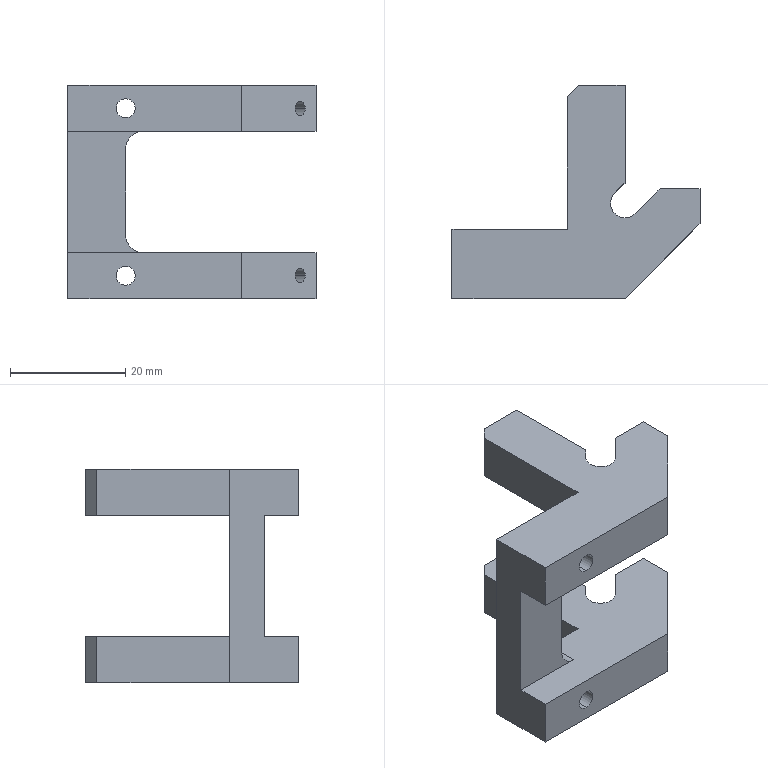Part | NX | features BREP 1 | 1 solid | 42 faces | box 43 x 37 x 37 mm | volume 12861 mm3 | plane 28 | cylinder 14 | commonest cylinder face diameters 2.5 x4 3.3 x4 5.05 x4 6 x2
STEP:
#1=CARTESIAN_POINT('',(-10.,0.,16.15));
#2=VERTEX_POINT('',#1);
#3=CARTESIAN_POINT('',(-10.,-12.,16.15));
#4=VERTEX_POINT('',#3);
#5=CARTESIAN_POINT('',(-10.,-12.,16.15));
#6=DIRECTION('',(0.,-1.,0.));
#7=VECTOR('',#6,1000.);
#8=LINE('',#5,#7);
#9=EDGE_CURVE('',#2,#4,#8,.T.);
#10=ORIENTED_EDGE('',*,*,#9,.F.);
#11=CARTESIAN_POINT('',(-10.,0.,12.85));
#12=VERTEX_POINT('',#11);
#13=CARTESIAN_POINT('',(-10.,0.,14.5));
#14=DIRECTION('',(0.,-1.,0.));
#15=DIRECTION('',(0.,0.,-1.));
#16=AXIS2_PLACEMENT_3D('',#13,#14,#15);
#17=CIRCLE('',#16,1.65);
#18=EDGE_CURVE('',#12,#2,#17,.T.);
#19=ORIENTED_EDGE('',*,*,#18,.F.);
#20=CARTESIAN_POINT('',(-10.,-12.,12.85));
#21=VERTEX_POINT('',#20);
#22=CARTESIAN_POINT('',(-10.,-12.,12.85));
#23=DIRECTION('',(0.,-1.,0.));
#24=VECTOR('',#23,1000.);
#25=LINE('',#22,#24);
#26=EDGE_CURVE('',#12,#21,#25,.T.);
#27=ORIENTED_EDGE('',*,*,#26,.T.);
#28=CARTESIAN_POINT('',(-10.,-12.,14.5));
#29=DIRECTION('',(0.,-1.,0.));
#30=DIRECTION('',(0.,0.,-1.));
#31=AXIS2_PLACEMENT_3D('',#28,#29,#30);
#32=CIRCLE('',#31,1.65);
#33=EDGE_CURVE('',#21,#4,#32,.T.);
#34=ORIENTED_EDGE('',*,*,#33,.T.);
#35=EDGE_LOOP('',(#10,#19,#27,#34));
#36=FACE_BOUND('',#35,.T.);
#37=CARTESIAN_POINT('',(-10.,-12.,14.5));
#38=DIRECTION('',(0.,-1.,0.));
#39=DIRECTION('',(0.,0.,-1.));
#40=AXIS2_PLACEMENT_3D('',#37,#38,#39);
#41=CYLINDRICAL_SURFACE('',#40,1.65);
#42=ADVANCED_FACE('',(#36),#41,.F.);
#43=CARTESIAN_POINT('',(-10.,0.,-12.85));
#44=VERTEX_POINT('',#43);
#45=CARTESIAN_POINT('',(-10.,-12.,-12.85));
#46=VERTEX_POINT('',#45);
#47=CARTESIAN_POINT('',(-10.,-12.,-12.85));
#48=DIRECTION('',(0.,-1.,0.));
#49=VECTOR('',#48,1000.);
#50=LINE('',#47,#49);
#51=EDGE_CURVE('',#44,#46,#50,.T.);
#52=ORIENTED_EDGE('',*,*,#51,.F.);
#53=CARTESIAN_POINT('',(-10.,0.,-16.15));
#54=VERTEX_POINT('',#53);
#55=CARTESIAN_POINT('',(-10.,0.,-14.5));
#56=DIRECTION('',(0.,-1.,0.));
#57=DIRECTION('',(0.,0.,-1.));
#58=AXIS2_PLACEMENT_3D('',#55,#56,#57);
#59=CIRCLE('',#58,1.65);
#60=EDGE_CURVE('',#54,#44,#59,.T.);
#61=ORIENTED_EDGE('',*,*,#60,.F.);
#62=CARTESIAN_POINT('',(-10.,-12.,-16.15));
#63=VERTEX_POINT('',#62);
#64=CARTESIAN_POINT('',(-10.,-12.,-16.15));
#65=DIRECTION('',(0.,-1.,0.));
#66=VECTOR('',#65,1000.);
#67=LINE('',#64,#66);
#68=EDGE_CURVE('',#54,#63,#67,.T.);
#69=ORIENTED_EDGE('',*,*,#68,.T.);
#70=CARTESIAN_POINT('',(-10.,-12.,-14.5));
#71=DIRECTION('',(0.,-1.,0.));
#72=DIRECTION('',(0.,0.,-1.));
#73=AXIS2_PLACEMENT_3D('',#70,#71,#72);
#74=CIRCLE('',#73,1.65);
#75=EDGE_CURVE('',#63,#46,#74,.T.);
#76=ORIENTED_EDGE('',*,*,#75,.T.);
#77=EDGE_LOOP('',(#52,#61,#69,#76));
#78=FACE_BOUND('',#77,.T.);
#79=CARTESIAN_POINT('',(-10.,-12.,-14.5));
#80=DIRECTION('',(0.,-1.,0.));
#81=DIRECTION('',(0.,0.,-1.));
#82=AXIS2_PLACEMENT_3D('',#79,#80,#81);
#83=CYLINDRICAL_SURFACE('',#82,1.65);
#84=ADVANCED_FACE('',(#78),#83,.F.);
#85=CARTESIAN_POINT('',(-10.,-6.,7.5));
#86=VERTEX_POINT('',#85);
#87=CARTESIAN_POINT('',(-7.,-6.,10.5));
#88=VERTEX_POINT('',#87);
#89=CARTESIAN_POINT('',(-7.,-6.,7.5));
#90=DIRECTION('',(0.,1.,0.));
#91=DIRECTION('',(1.,0.,0.));
#92=AXIS2_PLACEMENT_3D('',#89,#90,#91);
#93=CIRCLE('',#92,3.);
#94=EDGE_CURVE('',#86,#88,#93,.T.);
#95=ORIENTED_EDGE('',*,*,#94,.T.);
#96=CARTESIAN_POINT('',(-20.,-6.,10.5));
#97=VERTEX_POINT('',#96);
#98=CARTESIAN_POINT('',(-20.,-6.,10.5));
#99=DIRECTION('',(-1.,0.,0.));
#100=VECTOR('',#99,1000.);
#101=LINE('',#98,#100);
#102=EDGE_CURVE('',#88,#97,#101,.T.);
#103=ORIENTED_EDGE('',*,*,#102,.T.);
#104=CARTESIAN_POINT('',(-20.,-6.,-10.5));
#105=VERTEX_POINT('',#104);
#106=CARTESIAN_POINT('',(-20.,-6.,10.5));
#107=DIRECTION('',(0.,0.,-1.));
#108=VECTOR('',#107,1000.);
#109=LINE('',#106,#108);
#110=EDGE_CURVE('',#97,#105,#109,.T.);
#111=ORIENTED_EDGE('',*,*,#110,.T.);
#112=CARTESIAN_POINT('',(-7.,-6.,-10.5));
#113=VERTEX_POINT('',#112);
#114=CARTESIAN_POINT('',(-20.,-6.,-10.5));
#115=DIRECTION('',(1.,0.,0.));
#116=VECTOR('',#115,1000.);
#117=LINE('',#114,#116);
#118=EDGE_CURVE('',#105,#113,#117,.T.);
#119=ORIENTED_EDGE('',*,*,#118,.T.);
#120=CARTESIAN_POINT('',(-10.,-6.,-7.5));
#121=VERTEX_POINT('',#120);
#122=CARTESIAN_POINT('',(-7.,-6.,-7.5));
#123=DIRECTION('',(0.,1.,0.));
#124=DIRECTION('',(1.,0.,0.));
#125=AXIS2_PLACEMENT_3D('',#122,#123,#124);
#126=CIRCLE('',#125,3.);
#127=EDGE_CURVE('',#113,#121,#126,.T.);
#128=ORIENTED_EDGE('',*,*,#127,.T.);
#129=CARTESIAN_POINT('',(-10.,-6.,-7.5));
#130=DIRECTION('',(0.,0.,1.));
#131=VECTOR('',#130,1000.);
#132=LINE('',#129,#131);
#133=EDGE_CURVE('',#121,#86,#132,.T.);
#134=ORIENTED_EDGE('',*,*,#133,.T.);
#135=EDGE_LOOP('',(#95,#103,#111,#119,#128,#134));
#136=FACE_BOUND('',#135,.T.);
#137=CARTESIAN_POINT('',(0.,-6.,0.));
#138=DIRECTION('',(0.,-1.,0.));
#139=DIRECTION('',(1.,0.,0.));
#140=AXIS2_PLACEMENT_3D('',#137,#138,#139);
#141=PLANE('',#140);
#142=ADVANCED_FACE('',(#136),#141,.T.);
#143=CARTESIAN_POINT('',(2.,25.,-10.5));
#144=VERTEX_POINT('',#143);
#145=CARTESIAN_POINT('',(0.,23.,-10.5));
#146=VERTEX_POINT('',#145);
#147=CARTESIAN_POINT('',(0.,23.,-10.5));
#148=DIRECTION('',(-0.7071,-0.7071,0.));
#149=VECTOR('',#148,1000.);
#150=LINE('',#147,#149);
#151=EDGE_CURVE('',#144,#146,#150,.T.);
#152=ORIENTED_EDGE('',*,*,#151,.F.);
#153=CARTESIAN_POINT('',(2.,25.,-18.5));
#154=VERTEX_POINT('',#153);
#155=CARTESIAN_POINT('',(2.,25.,18.5));
#156=DIRECTION('',(0.,0.,1.));
#157=VECTOR('',#156,1000.);
#158=LINE('',#155,#157);
#159=EDGE_CURVE('',#154,#144,#158,.T.);
#160=ORIENTED_EDGE('',*,*,#159,.F.);
#161=CARTESIAN_POINT('',(0.,23.,-18.5));
#162=VERTEX_POINT('',#161);
#163=CARTESIAN_POINT('',(0.,23.,-18.5));
#164=DIRECTION('',(0.7071,0.7071,0.));
#165=VECTOR('',#164,1000.);
#166=LINE('',#163,#165);
#167=EDGE_CURVE('',#162,#154,#166,.T.);
#168=ORIENTED_EDGE('',*,*,#167,.F.);
#169=CARTESIAN_POINT('',(0.,23.,18.5));
#170=DIRECTION('',(0.,0.,-1.));
#171=VECTOR('',#170,1000.);
#172=LINE('',#169,#171);
#173=EDGE_CURVE('',#146,#162,#172,.T.);
#174=ORIENTED_EDGE('',*,*,#173,.F.);
#175=EDGE_LOOP('',(#152,#160,#168,#174));
#176=FACE_BOUND('',#175,.T.);
#177=CARTESIAN_POINT('',(0.,23.,18.5));
#178=DIRECTION('',(0.7071,-0.7071,0.));
#179=DIRECTION('',(0.,0.,-1.));
#180=AXIS2_PLACEMENT_3D('',#177,#178,#179);
#181=PLANE('',#180);
#182=ADVANCED_FACE('',(#176),#181,.F.);
#183=CARTESIAN_POINT('',(2.,25.,18.5));
#184=VERTEX_POINT('',#183);
#185=CARTESIAN_POINT('',(0.,23.,18.5));
#186=VERTEX_POINT('',#185);
#187=CARTESIAN_POINT('',(-4.25,18.75,18.5));
#188=DIRECTION('',(-0.7071,-0.7071,0.));
#189=VECTOR('',#188,1000.);
#190=LINE('',#187,#189);
#191=EDGE_CURVE('',#184,#186,#190,.T.);
#192=ORIENTED_EDGE('',*,*,#191,.F.);
#193=CARTESIAN_POINT('',(2.,25.,10.5));
#194=VERTEX_POINT('',#193);
#195=CARTESIAN_POINT('',(2.,25.,18.5));
#196=DIRECTION('',(0.,0.,1.));
#197=VECTOR('',#196,1000.);
#198=LINE('',#195,#197);
#199=EDGE_CURVE('',#194,#184,#198,.T.);
#200=ORIENTED_EDGE('',*,*,#199,.F.);
#201=CARTESIAN_POINT('',(0.,23.,10.5));
#202=VERTEX_POINT('',#201);
#203=CARTESIAN_POINT('',(0.,23.,10.5));
#204=DIRECTION('',(0.7071,0.7071,0.));
#205=VECTOR('',#204,1000.);
#206=LINE('',#203,#205);
#207=EDGE_CURVE('',#202,#194,#206,.T.);
#208=ORIENTED_EDGE('',*,*,#207,.F.);
#209=CARTESIAN_POINT('',(0.,23.,18.5));
#210=DIRECTION('',(0.,0.,-1.));
#211=VECTOR('',#210,1000.);
#212=LINE('',#209,#211);
#213=EDGE_CURVE('',#186,#202,#212,.T.);
#214=ORIENTED_EDGE('',*,*,#213,.F.);
#215=EDGE_LOOP('',(#192,#200,#208,#214));
#216=FACE_BOUND('',#215,.T.);
#217=CARTESIAN_POINT('',(0.,23.,18.5));
#218=DIRECTION('',(0.7071,-0.7071,0.));
#219=DIRECTION('',(0.,0.,-1.));
#220=AXIS2_PLACEMENT_3D('',#217,#218,#219);
#221=PLANE('',#220);
#222=ADVANCED_FACE('',(#216),#221,.F.);
#223=CARTESIAN_POINT('',(19.369,-2.631,-14.5));
#224=VERTEX_POINT('',#223);
#225=CARTESIAN_POINT('',(12.905,3.834,-14.5));
#226=VERTEX_POINT('',#225);
#227=CARTESIAN_POINT('',(19.369,-2.631,-14.5));
#228=DIRECTION('',(0.7071,-0.7071,0.));
#229=VECTOR('',#228,1000.);
#230=LINE('',#227,#229);
#231=EDGE_CURVE('',#224,#226,#230,.F.);
#232=ORIENTED_EDGE('',*,*,#231,.T.);
#233=CARTESIAN_POINT('',(14.672,5.601,-14.5));
#234=VERTEX_POINT('',#233);
#235=CARTESIAN_POINT('',(13.788,4.718,-14.5));
#236=DIRECTION('',(0.7071,-0.7071,0.));
#237=DIRECTION('',(0.7071,0.7071,0.));
#238=AXIS2_PLACEMENT_3D('',#235,#236,#237);
#239=CIRCLE('',#238,1.25);
#240=EDGE_CURVE('',#234,#226,#239,.T.);
#241=ORIENTED_EDGE('',*,*,#240,.F.);
#242=CARTESIAN_POINT('',(21.137,-0.8631,-14.5));
#243=VERTEX_POINT('',#242);
#244=CARTESIAN_POINT('',(21.137,-0.8631,-14.5));
#245=DIRECTION('',(0.7071,-0.7071,0.));
#246=VECTOR('',#245,1000.);
#247=LINE('',#244,#246);
#248=EDGE_CURVE('',#243,#234,#247,.F.);
#249=ORIENTED_EDGE('',*,*,#248,.F.);
#250=CARTESIAN_POINT('',(20.253,-1.747,-14.5));
#251=DIRECTION('',(0.7071,-0.7071,0.));
#252=DIRECTION('',(0.7071,0.7071,0.));
#253=AXIS2_PLACEMENT_3D('',#250,#251,#252);
#254=CIRCLE('',#253,1.25);
#255=EDGE_CURVE('',#243,#224,#254,.T.);
#256=ORIENTED_EDGE('',*,*,#255,.T.);
#257=EDGE_LOOP('',(#232,#241,#249,#256));
#258=FACE_BOUND('',#257,.T.);
#259=CARTESIAN_POINT('',(20.253,-1.747,-14.5));
#260=DIRECTION('',(0.7071,-0.7071,0.));
#261=DIRECTION('',(0.7071,0.7071,0.));
#262=AXIS2_PLACEMENT_3D('',#259,#260,#261);
#263=CYLINDRICAL_SURFACE('',#262,1.25);
#264=ADVANCED_FACE('',(#258),#263,.F.);
#265=CARTESIAN_POINT('',(19.369,-2.631,14.5));
#266=VERTEX_POINT('',#265);
#267=CARTESIAN_POINT('',(12.905,3.834,14.5));
#268=VERTEX_POINT('',#267);
#269=CARTESIAN_POINT('',(19.369,-2.631,14.5));
#270=DIRECTION('',(0.7071,-0.7071,0.));
#271=VECTOR('',#270,1000.);
#272=LINE('',#269,#271);
#273=EDGE_CURVE('',#266,#268,#272,.F.);
#274=ORIENTED_EDGE('',*,*,#273,.T.);
#275=CARTESIAN_POINT('',(14.672,5.601,14.5));
#276=VERTEX_POINT('',#275);
#277=CARTESIAN_POINT('',(13.788,4.718,14.5));
#278=DIRECTION('',(0.7071,-0.7071,0.));
#279=DIRECTION('',(0.7071,0.7071,0.));
#280=AXIS2_PLACEMENT_3D('',#277,#278,#279);
#281=CIRCLE('',#280,1.25);
#282=EDGE_CURVE('',#276,#268,#281,.T.);
#283=ORIENTED_EDGE('',*,*,#282,.F.);
#284=CARTESIAN_POINT('',(21.137,-0.8631,14.5));
#285=VERTEX_POINT('',#284);
#286=CARTESIAN_POINT('',(21.137,-0.8631,14.5));
#287=DIRECTION('',(0.7071,-0.7071,0.));
#288=VECTOR('',#287,1000.);
#289=LINE('',#286,#288);
#290=EDGE_CURVE('',#285,#276,#289,.F.);
#291=ORIENTED_EDGE('',*,*,#290,.F.);
#292=CARTESIAN_POINT('',(20.253,-1.747,14.5));
#293=DIRECTION('',(0.7071,-0.7071,0.));
#294=DIRECTION('',(0.7071,0.7071,0.));
#295=AXIS2_PLACEMENT_3D('',#292,#293,#294);
#296=CIRCLE('',#295,1.25);
#297=EDGE_CURVE('',#285,#266,#296,.T.);
#298=ORIENTED_EDGE('',*,*,#297,.T.);
#299=EDGE_LOOP('',(#274,#283,#291,#298));
#300=FACE_BOUND('',#299,.T.);
#301=CARTESIAN_POINT('',(20.253,-1.747,14.5));
#302=DIRECTION('',(0.7071,-0.7071,0.));
#303=DIRECTION('',(0.7071,0.7071,0.));
#304=AXIS2_PLACEMENT_3D('',#301,#302,#303);
#305=CYLINDRICAL_SURFACE('',#304,1.25);
#306=ADVANCED_FACE('',(#300),#305,.F.);
#307=CARTESIAN_POINT('',(-20.,-12.,-10.5));
#308=VERTEX_POINT('',#307);
#309=CARTESIAN_POINT('',(-20.,-6.,-10.5));
#310=DIRECTION('',(0.,-1.,0.));
#311=VECTOR('',#310,1000.);
#312=LINE('',#309,#311);
#313=EDGE_CURVE('',#105,#308,#312,.T.);
#314=ORIENTED_EDGE('',*,*,#313,.T.);
#315=CARTESIAN_POINT('',(10.,-12.,-10.5));
#316=VERTEX_POINT('',#315);
#317=CARTESIAN_POINT('',(56.,-12.,-10.5));
#318=DIRECTION('',(-1.,0.,0.));
#319=VECTOR('',#318,1000.);
#320=LINE('',#317,#319);
#321=EDGE_CURVE('',#316,#308,#320,.T.);
#322=ORIENTED_EDGE('',*,*,#321,.F.);
#323=CARTESIAN_POINT('',(23.,1.,-10.5));
#324=VERTEX_POINT('',#323);
#325=CARTESIAN_POINT('',(23.,1.,-10.5));
#326=DIRECTION('',(-0.7071,-0.7071,0.));
#327=VECTOR('',#326,1000.);
#328=LINE('',#325,#327);
#329=EDGE_CURVE('',#324,#316,#328,.T.);
#330=ORIENTED_EDGE('',*,*,#329,.F.);
#331=CARTESIAN_POINT('',(23.,7.,-10.5));
#332=VERTEX_POINT('',#331);
#333=CARTESIAN_POINT('',(23.,7.,-10.5));
#334=DIRECTION('',(0.,-1.,0.));
#335=VECTOR('',#334,1000.);
#336=LINE('',#333,#335);
#337=EDGE_CURVE('',#332,#324,#336,.T.);
#338=ORIENTED_EDGE('',*,*,#337,.F.);
#339=CARTESIAN_POINT('',(16.071,7.,-10.5));
#340=VERTEX_POINT('',#339);
#341=CARTESIAN_POINT('',(16.071,7.,-10.5));
#342=DIRECTION('',(1.,0.,0.));
#343=VECTOR('',#342,1000.);
#344=LINE('',#341,#343);
#345=EDGE_CURVE('',#340,#332,#344,.T.);
#346=ORIENTED_EDGE('',*,*,#345,.F.);
#347=CARTESIAN_POINT('',(11.785,2.715,-10.5));
#348=VERTEX_POINT('',#347);
#349=CARTESIAN_POINT('',(11.785,2.715,-10.5));
#350=DIRECTION('',(0.7071,0.7071,0.));
#351=VECTOR('',#350,1000.);
#352=LINE('',#349,#351);
#353=EDGE_CURVE('',#348,#340,#352,.T.);
#354=ORIENTED_EDGE('',*,*,#353,.F.);
#355=CARTESIAN_POINT('',(7.475,4.5,-10.5));
#356=VERTEX_POINT('',#355);
#357=CARTESIAN_POINT('',(10.,4.5,-10.5));
#358=DIRECTION('',(0.,0.,1.));
#359=DIRECTION('',(-1.,0.,0.));
#360=AXIS2_PLACEMENT_3D('',#357,#358,#359);
#361=CIRCLE('',#360,2.525);
#362=EDGE_CURVE('',#356,#348,#361,.T.);
#363=ORIENTED_EDGE('',*,*,#362,.F.);
#364=CARTESIAN_POINT('',(8.215,6.285,-10.5));
#365=VERTEX_POINT('',#364);
#366=CARTESIAN_POINT('',(10.,4.5,-10.5));
#367=DIRECTION('',(0.,0.,1.));
#368=DIRECTION('',(-1.,0.,0.));
#369=AXIS2_PLACEMENT_3D('',#366,#367,#368);
#370=CIRCLE('',#369,2.525);
#371=EDGE_CURVE('',#365,#356,#370,.T.);
#372=ORIENTED_EDGE('',*,*,#371,.F.);
#373=CARTESIAN_POINT('',(10.,8.071,-10.5));
#374=VERTEX_POINT('',#373);
#375=CARTESIAN_POINT('',(8.215,6.285,-10.5));
#376=DIRECTION('',(-0.7071,-0.7071,0.));
#377=VECTOR('',#376,1000.);
#378=LINE('',#375,#377);
#379=EDGE_CURVE('',#374,#365,#378,.T.);
#380=ORIENTED_EDGE('',*,*,#379,.F.);
#381=CARTESIAN_POINT('',(10.,25.,-10.5));
#382=VERTEX_POINT('',#381);
#383=CARTESIAN_POINT('',(10.,25.,-10.5));
#384=DIRECTION('',(0.,-1.,0.));
#385=VECTOR('',#384,1000.);
#386=LINE('',#383,#385);
#387=EDGE_CURVE('',#382,#374,#386,.T.);
#388=ORIENTED_EDGE('',*,*,#387,.F.);
#389=CARTESIAN_POINT('',(56.,25.,-10.5));
#390=DIRECTION('',(-1.,0.,0.));
#391=VECTOR('',#390,1000.);
#392=LINE('',#389,#391);
#393=EDGE_CURVE('',#382,#144,#392,.T.);
#394=ORIENTED_EDGE('',*,*,#393,.T.);
#395=ORIENTED_EDGE('',*,*,#151,.T.);
#396=CARTESIAN_POINT('',(0.,0.,-10.5));
#397=VERTEX_POINT('',#396);
#398=CARTESIAN_POINT('',(0.,0.,-10.5));
#399=DIRECTION('',(0.,1.,0.));
#400=VECTOR('',#399,1000.);
#401=LINE('',#398,#400);
#402=EDGE_CURVE('',#397,#146,#401,.T.);
#403=ORIENTED_EDGE('',*,*,#402,.F.);
#404=CARTESIAN_POINT('',(-7.,0.,-10.5));
#405=VERTEX_POINT('',#404);
#406=CARTESIAN_POINT('',(-20.,0.,-10.5));
#407=DIRECTION('',(1.,0.,0.));
#408=VECTOR('',#407,1000.);
#409=LINE('',#406,#408);
#410=EDGE_CURVE('',#405,#397,#409,.T.);
#411=ORIENTED_EDGE('',*,*,#410,.F.);
#412=CARTESIAN_POINT('',(-7.,-12.,-10.5));
#413=DIRECTION('',(0.,1.,0.));
#414=VECTOR('',#413,1000.);
#415=LINE('',#412,#414);
#416=EDGE_CURVE('',#113,#405,#415,.T.);
#417=ORIENTED_EDGE('',*,*,#416,.F.);
#418=ORIENTED_EDGE('',*,*,#118,.F.);
#419=EDGE_LOOP('',(#314,#322,#330,#338,#346,#354,#363,#372,#380,#388,#394,#395,#403,#411,#417,#418));
#420=FACE_BOUND('',#419,.T.);
#421=CARTESIAN_POINT('',(56.,-12.,-10.5));
#422=DIRECTION('',(0.,0.,-1.));
#423=DIRECTION('',(-1.,0.,0.));
#424=AXIS2_PLACEMENT_3D('',#421,#422,#423);
#425=PLANE('',#424);
#426=ADVANCED_FACE('',(#420),#425,.F.);
#427=CARTESIAN_POINT('',(10.,-12.,10.5));
#428=VERTEX_POINT('',#427);
#429=CARTESIAN_POINT('',(23.,1.,10.5));
#430=VERTEX_POINT('',#429);
#431=CARTESIAN_POINT('',(23.,1.,10.5));
#432=DIRECTION('',(0.7071,0.7071,0.));
#433=VECTOR('',#432,1000.);
#434=LINE('',#431,#433);
#435=EDGE_CURVE('',#428,#430,#434,.T.);
#436=ORIENTED_EDGE('',*,*,#435,.F.);
#437=CARTESIAN_POINT('',(-20.,-12.,10.5));
#438=VERTEX_POINT('',#437);
#439=CARTESIAN_POINT('',(56.,-12.,10.5));
#440=DIRECTION('',(1.,0.,0.));
#441=VECTOR('',#440,1000.);
#442=LINE('',#439,#441);
#443=EDGE_CURVE('',#438,#428,#442,.T.);
#444=ORIENTED_EDGE('',*,*,#443,.F.);
#445=CARTESIAN_POINT('',(-20.,-6.,10.5));
#446=DIRECTION('',(0.,-1.,0.));
#447=VECTOR('',#446,1000.);
#448=LINE('',#445,#447);
#449=EDGE_CURVE('',#97,#438,#448,.T.);
#450=ORIENTED_EDGE('',*,*,#449,.F.);
#451=ORIENTED_EDGE('',*,*,#102,.F.);
#452=CARTESIAN_POINT('',(-7.,0.,10.5));
#453=VERTEX_POINT('',#452);
#454=CARTESIAN_POINT('',(-7.,-12.,10.5));
#455=DIRECTION('',(0.,1.,0.));
#456=VECTOR('',#455,1000.);
#457=LINE('',#454,#456);
#458=EDGE_CURVE('',#88,#453,#457,.T.);
#459=ORIENTED_EDGE('',*,*,#458,.T.);
#460=CARTESIAN_POINT('',(0.,0.,10.5));
#461=VERTEX_POINT('',#460);
#462=CARTESIAN_POINT('',(-20.,0.,10.5));
#463=DIRECTION('',(-1.,0.,0.));
#464=VECTOR('',#463,1000.);
#465=LINE('',#462,#464);
#466=EDGE_CURVE('',#461,#453,#465,.T.);
#467=ORIENTED_EDGE('',*,*,#466,.F.);
#468=CARTESIAN_POINT('',(0.,0.,10.5));
#469=DIRECTION('',(0.,-1.,0.));
#470=VECTOR('',#469,1000.);
#471=LINE('',#468,#470);
#472=EDGE_CURVE('',#202,#461,#471,.T.);
#473=ORIENTED_EDGE('',*,*,#472,.F.);
#474=ORIENTED_EDGE('',*,*,#207,.T.);
#475=CARTESIAN_POINT('',(10.,25.,10.5));
#476=VERTEX_POINT('',#475);
#477=CARTESIAN_POINT('',(56.,25.,10.5));
#478=DIRECTION('',(1.,0.,0.));
#479=VECTOR('',#478,1000.);
#480=LINE('',#477,#479);
#481=EDGE_CURVE('',#194,#476,#480,.T.);
#482=ORIENTED_EDGE('',*,*,#481,.T.);
#483=CARTESIAN_POINT('',(10.,8.071,10.5));
#484=VERTEX_POINT('',#483);
#485=CARTESIAN_POINT('',(10.,25.,10.5));
#486=DIRECTION('',(0.,1.,0.));
#487=VECTOR('',#486,1000.);
#488=LINE('',#485,#487);
#489=EDGE_CURVE('',#484,#476,#488,.T.);
#490=ORIENTED_EDGE('',*,*,#489,.F.);
#491=CARTESIAN_POINT('',(8.215,6.285,10.5));
#492=VERTEX_POINT('',#491);
#493=CARTESIAN_POINT('',(8.215,6.285,10.5));
#494=DIRECTION('',(0.7071,0.7071,0.));
#495=VECTOR('',#494,1000.);
#496=LINE('',#493,#495);
#497=EDGE_CURVE('',#492,#484,#496,.T.);
#498=ORIENTED_EDGE('',*,*,#497,.F.);
#499=CARTESIAN_POINT('',(7.475,4.5,10.5));
#500=VERTEX_POINT('',#499);
#501=CARTESIAN_POINT('',(10.,4.5,10.5));
#502=DIRECTION('',(0.,0.,-1.));
#503=DIRECTION('',(1.,0.,0.));
#504=AXIS2_PLACEMENT_3D('',#501,#502,#503);
#505=CIRCLE('',#504,2.525);
#506=EDGE_CURVE('',#500,#492,#505,.T.);
#507=ORIENTED_EDGE('',*,*,#506,.F.);
#508=CARTESIAN_POINT('',(11.785,2.715,10.5));
#509=VERTEX_POINT('',#508);
#510=CARTESIAN_POINT('',(10.,4.5,10.5));
#511=DIRECTION('',(0.,0.,-1.));
#512=DIRECTION('',(1.,0.,0.));
#513=AXIS2_PLACEMENT_3D('',#510,#511,#512);
#514=CIRCLE('',#513,2.525);
#515=EDGE_CURVE('',#509,#500,#514,.T.);
#516=ORIENTED_EDGE('',*,*,#515,.F.);
#517=CARTESIAN_POINT('',(16.071,7.,10.5));
#518=VERTEX_POINT('',#517);
#519=CARTESIAN_POINT('',(11.785,2.715,10.5));
#520=DIRECTION('',(-0.7071,-0.7071,0.));
#521=VECTOR('',#520,1000.);
#522=LINE('',#519,#521);
#523=EDGE_CURVE('',#518,#509,#522,.T.);
#524=ORIENTED_EDGE('',*,*,#523,.F.);
#525=CARTESIAN_POINT('',(23.,7.,10.5));
#526=VERTEX_POINT('',#525);
#527=CARTESIAN_POINT('',(16.071,7.,10.5));
#528=DIRECTION('',(-1.,0.,0.));
#529=VECTOR('',#528,1000.);
#530=LINE('',#527,#529);
#531=EDGE_CURVE('',#526,#518,#530,.T.);
#532=ORIENTED_EDGE('',*,*,#531,.F.);
#533=CARTESIAN_POINT('',(23.,7.,10.5));
#534=DIRECTION('',(0.,1.,0.));
#535=VECTOR('',#534,1000.);
#536=LINE('',#533,#535);
#537=EDGE_CURVE('',#430,#526,#536,.T.);
#538=ORIENTED_EDGE('',*,*,#537,.F.);
#539=EDGE_LOOP('',(#436,#444,#450,#451,#459,#467,#473,#474,#482,#490,#498,#507,#516,#524,#532,#538));
#540=FACE_BOUND('',#539,.T.);
#541=CARTESIAN_POINT('',(56.,-12.,10.5));
#542=DIRECTION('',(0.,0.,1.));
#543=DIRECTION('',(1.,0.,0.));
#544=AXIS2_PLACEMENT_3D('',#541,#542,#543);
#545=PLANE('',#544);
#546=ADVANCED_FACE('',(#540),#545,.F.);
#547=CARTESIAN_POINT('',(0.,0.,-18.5));
#548=VERTEX_POINT('',#547);
#549=CARTESIAN_POINT('',(0.,0.,-18.5));
#550=DIRECTION('',(0.,-1.,0.));
#551=VECTOR('',#550,1000.);
#552=LINE('',#549,#551);
#553=EDGE_CURVE('',#162,#548,#552,.T.);
#554=ORIENTED_EDGE('',*,*,#553,.F.);
#555=ORIENTED_EDGE('',*,*,#167,.T.);
#556=CARTESIAN_POINT('',(10.,25.,-18.5));
#557=VERTEX_POINT('',#556);
#558=CARTESIAN_POINT('',(0.,25.,-18.5));
#559=DIRECTION('',(-1.,0.,0.));
#560=VECTOR('',#559,1000.);
#561=LINE('',#558,#560);
#562=EDGE_CURVE('',#557,#154,#561,.T.);
#563=ORIENTED_EDGE('',*,*,#562,.F.);
#564=CARTESIAN_POINT('',(10.,8.071,-18.5));
#565=VERTEX_POINT('',#564);
#566=CARTESIAN_POINT('',(10.,25.,-18.5));
#567=DIRECTION('',(0.,1.,0.));
#568=VECTOR('',#567,1000.);
#569=LINE('',#566,#568);
#570=EDGE_CURVE('',#565,#557,#569,.T.);
#571=ORIENTED_EDGE('',*,*,#570,.F.);
#572=CARTESIAN_POINT('',(8.215,6.285,-18.5));
#573=VERTEX_POINT('',#572);
#574=CARTESIAN_POINT('',(8.215,6.285,-18.5));
#575=DIRECTION('',(0.7071,0.7071,0.));
#576=VECTOR('',#575,1000.);
#577=LINE('',#574,#576);
#578=EDGE_CURVE('',#573,#565,#577,.T.);
#579=ORIENTED_EDGE('',*,*,#578,.F.);
#580=CARTESIAN_POINT('',(7.475,4.5,-18.5));
#581=VERTEX_POINT('',#580);
#582=CARTESIAN_POINT('',(10.,4.5,-18.5));
#583=DIRECTION('',(0.,0.,-1.));
#584=DIRECTION('',(1.,0.,0.));
#585=AXIS2_PLACEMENT_3D('',#582,#583,#584);
#586=CIRCLE('',#585,2.525);
#587=EDGE_CURVE('',#581,#573,#586,.T.);
#588=ORIENTED_EDGE('',*,*,#587,.F.);
#589=CARTESIAN_POINT('',(11.785,2.715,-18.5));
#590=VERTEX_POINT('',#589);
#591=CARTESIAN_POINT('',(10.,4.5,-18.5));
#592=DIRECTION('',(0.,0.,-1.));
#593=DIRECTION('',(1.,0.,0.));
#594=AXIS2_PLACEMENT_3D('',#591,#592,#593);
#595=CIRCLE('',#594,2.525);
#596=EDGE_CURVE('',#590,#581,#595,.T.);
#597=ORIENTED_EDGE('',*,*,#596,.F.);
#598=CARTESIAN_POINT('',(16.071,7.,-18.5));
#599=VERTEX_POINT('',#598);
#600=CARTESIAN_POINT('',(11.785,2.715,-18.5));
#601=DIRECTION('',(-0.7071,-0.7071,0.));
#602=VECTOR('',#601,1000.);
#603=LINE('',#600,#602);
#604=EDGE_CURVE('',#599,#590,#603,.T.);
#605=ORIENTED_EDGE('',*,*,#604,.F.);
#606=CARTESIAN_POINT('',(23.,7.,-18.5));
#607=VERTEX_POINT('',#606);
#608=CARTESIAN_POINT('',(16.071,7.,-18.5));
#609=DIRECTION('',(-1.,0.,0.));
#610=VECTOR('',#609,1000.);
#611=LINE('',#608,#610);
#612=EDGE_CURVE('',#607,#599,#611,.T.);
#613=ORIENTED_EDGE('',*,*,#612,.F.);
#614=CARTESIAN_POINT('',(23.,1.,-18.5));
#615=VERTEX_POINT('',#614);
#616=CARTESIAN_POINT('',(23.,7.,-18.5));
#617=DIRECTION('',(0.,1.,0.));
#618=VECTOR('',#617,1000.);
#619=LINE('',#616,#618);
#620=EDGE_CURVE('',#615,#607,#619,.T.);
#621=ORIENTED_EDGE('',*,*,#620,.F.);
#622=CARTESIAN_POINT('',(10.,-12.,-18.5));
#623=VERTEX_POINT('',#622);
#624=CARTESIAN_POINT('',(23.,1.,-18.5));
#625=DIRECTION('',(0.7071,0.7071,0.));
#626=VECTOR('',#625,1000.);
#627=LINE('',#624,#626);
#628=EDGE_CURVE('',#623,#615,#627,.T.);
#629=ORIENTED_EDGE('',*,*,#628,.F.);
#630=CARTESIAN_POINT('',(-20.,-12.,-18.5));
#631=VERTEX_POINT('',#630);
#632=CARTESIAN_POINT('',(10.,-12.,-18.5));
#633=DIRECTION('',(1.,0.,0.));
#634=VECTOR('',#633,1000.);
#635=LINE('',#632,#634);
#636=EDGE_CURVE('',#631,#623,#635,.T.);
#637=ORIENTED_EDGE('',*,*,#636,.F.);
#638=CARTESIAN_POINT('',(-20.,0.,-18.5));
#639=VERTEX_POINT('',#638);
#640=CARTESIAN_POINT('',(-20.,-12.,-18.5));
#641=DIRECTION('',(0.,-1.,0.));
#642=VECTOR('',#641,1000.);
#643=LINE('',#640,#642);
#644=EDGE_CURVE('',#639,#631,#643,.T.);
#645=ORIENTED_EDGE('',*,*,#644,.F.);
#646=CARTESIAN_POINT('',(-20.,0.,-18.5));
#647=DIRECTION('',(-1.,0.,0.));
#648=VECTOR('',#647,1000.);
#649=LINE('',#646,#648);
#650=EDGE_CURVE('',#548,#639,#649,.T.);
#651=ORIENTED_EDGE('',*,*,#650,.F.);
#652=EDGE_LOOP('',(#554,#555,#563,#571,#579,#588,#597,#605,#613,#621,#629,#637,#645,#651));
#653=FACE_BOUND('',#652,.T.);
#654=CARTESIAN_POINT('',(10.,4.5,-18.5));
#655=DIRECTION('',(0.,0.,1.));
#656=DIRECTION('',(1.,0.,0.));
#657=AXIS2_PLACEMENT_3D('',#654,#655,#656);
#658=PLANE('',#657);
#659=ADVANCED_FACE('',(#653),#658,.F.);
#660=CARTESIAN_POINT('',(10.,25.,18.5));
#661=VERTEX_POINT('',#660);
#662=CARTESIAN_POINT('',(0.,25.,18.5));
#663=DIRECTION('',(-1.,0.,0.));
#664=VECTOR('',#663,1000.);
#665=LINE('',#662,#664);
#666=EDGE_CURVE('',#661,#184,#665,.T.);
#667=ORIENTED_EDGE('',*,*,#666,.T.);
#668=ORIENTED_EDGE('',*,*,#191,.T.);
#669=CARTESIAN_POINT('',(0.,0.,18.5));
#670=VERTEX_POINT('',#669);
#671=CARTESIAN_POINT('',(0.,0.,18.5));
#672=DIRECTION('',(0.,-1.,0.));
#673=VECTOR('',#672,1000.);
#674=LINE('',#671,#673);
#675=EDGE_CURVE('',#186,#670,#674,.T.);
#676=ORIENTED_EDGE('',*,*,#675,.T.);
#677=CARTESIAN_POINT('',(-20.,0.,18.5));
#678=VERTEX_POINT('',#677);
#679=CARTESIAN_POINT('',(-20.,0.,18.5));
#680=DIRECTION('',(-1.,0.,0.));
#681=VECTOR('',#680,1000.);
#682=LINE('',#679,#681);
#683=EDGE_CURVE('',#670,#678,#682,.T.);
#684=ORIENTED_EDGE('',*,*,#683,.T.);
#685=CARTESIAN_POINT('',(-20.,-12.,18.5));
#686=VERTEX_POINT('',#685);
#687=CARTESIAN_POINT('',(-20.,-12.,18.5));
#688=DIRECTION('',(0.,-1.,0.));
#689=VECTOR('',#688,1000.);
#690=LINE('',#687,#689);
#691=EDGE_CURVE('',#678,#686,#690,.T.);
#692=ORIENTED_EDGE('',*,*,#691,.T.);
#693=CARTESIAN_POINT('',(10.,-12.,18.5));
#694=VERTEX_POINT('',#693);
#695=CARTESIAN_POINT('',(10.,-12.,18.5));
#696=DIRECTION('',(1.,0.,0.));
#697=VECTOR('',#696,1000.);
#698=LINE('',#695,#697);
#699=EDGE_CURVE('',#686,#694,#698,.T.);
#700=ORIENTED_EDGE('',*,*,#699,.T.);
#701=CARTESIAN_POINT('',(23.,1.,18.5));
#702=VERTEX_POINT('',#701);
#703=CARTESIAN_POINT('',(23.,1.,18.5));
#704=DIRECTION('',(0.7071,0.7071,0.));
#705=VECTOR('',#704,1000.);
#706=LINE('',#703,#705);
#707=EDGE_CURVE('',#694,#702,#706,.T.);
#708=ORIENTED_EDGE('',*,*,#707,.T.);
#709=CARTESIAN_POINT('',(23.,7.,18.5));
#710=VERTEX_POINT('',#709);
#711=CARTESIAN_POINT('',(23.,7.,18.5));
#712=DIRECTION('',(0.,1.,0.));
#713=VECTOR('',#712,1000.);
#714=LINE('',#711,#713);
#715=EDGE_CURVE('',#702,#710,#714,.T.);
#716=ORIENTED_EDGE('',*,*,#715,.T.);
#717=CARTESIAN_POINT('',(16.071,7.,18.5));
#718=VERTEX_POINT('',#717);
#719=CARTESIAN_POINT('',(16.071,7.,18.5));
#720=DIRECTION('',(-1.,0.,0.));
#721=VECTOR('',#720,1000.);
#722=LINE('',#719,#721);
#723=EDGE_CURVE('',#710,#718,#722,.T.);
#724=ORIENTED_EDGE('',*,*,#723,.T.);
#725=CARTESIAN_POINT('',(11.785,2.715,18.5));
#726=VERTEX_POINT('',#725);
#727=CARTESIAN_POINT('',(11.785,2.715,18.5));
#728=DIRECTION('',(-0.7071,-0.7071,0.));
#729=VECTOR('',#728,1000.);
#730=LINE('',#727,#729);
#731=EDGE_CURVE('',#718,#726,#730,.T.);
#732=ORIENTED_EDGE('',*,*,#731,.T.);
#733=CARTESIAN_POINT('',(7.475,4.5,18.5));
#734=VERTEX_POINT('',#733);
#735=CARTESIAN_POINT('',(10.,4.5,18.5));
#736=DIRECTION('',(0.,0.,-1.));
#737=DIRECTION('',(1.,0.,0.));
#738=AXIS2_PLACEMENT_3D('',#735,#736,#737);
#739=CIRCLE('',#738,2.525);
#740=EDGE_CURVE('',#726,#734,#739,.T.);
#741=ORIENTED_EDGE('',*,*,#740,.T.);
#742=CARTESIAN_POINT('',(8.215,6.285,18.5));
#743=VERTEX_POINT('',#742);
#744=CARTESIAN_POINT('',(10.,4.5,18.5));
#745=DIRECTION('',(0.,0.,-1.));
#746=DIRECTION('',(1.,0.,0.));
#747=AXIS2_PLACEMENT_3D('',#744,#745,#746);
#748=CIRCLE('',#747,2.525);
#749=EDGE_CURVE('',#734,#743,#748,.T.);
#750=ORIENTED_EDGE('',*,*,#749,.T.);
#751=CARTESIAN_POINT('',(10.,8.071,18.5));
#752=VERTEX_POINT('',#751);
#753=CARTESIAN_POINT('',(8.215,6.285,18.5));
#754=DIRECTION('',(0.7071,0.7071,0.));
#755=VECTOR('',#754,1000.);
#756=LINE('',#753,#755);
#757=EDGE_CURVE('',#743,#752,#756,.T.);
#758=ORIENTED_EDGE('',*,*,#757,.T.);
#759=CARTESIAN_POINT('',(10.,25.,18.5));
#760=DIRECTION('',(0.,1.,0.));
#761=VECTOR('',#760,1000.);
#762=LINE('',#759,#761);
#763=EDGE_CURVE('',#752,#661,#762,.T.);
#764=ORIENTED_EDGE('',*,*,#763,.T.);
#765=EDGE_LOOP('',(#667,#668,#676,#684,#692,#700,#708,#716,#724,#732,#741,#750,#758,#764));
#766=FACE_BOUND('',#765,.T.);
#767=CARTESIAN_POINT('',(10.,4.5,18.5));
#768=DIRECTION('',(0.,0.,1.));
#769=DIRECTION('',(1.,0.,0.));
#770=AXIS2_PLACEMENT_3D('',#767,#768,#769);
#771=PLANE('',#770);
#772=ADVANCED_FACE('',(#766),#771,.T.);
#773=ORIENTED_EDGE('',*,*,#402,.T.);
#774=ORIENTED_EDGE('',*,*,#173,.T.);
#775=ORIENTED_EDGE('',*,*,#553,.T.);
#776=CARTESIAN_POINT('',(0.,0.,18.5));
#777=DIRECTION('',(0.,0.,-1.));
#778=VECTOR('',#777,1000.);
#779=LINE('',#776,#778);
#780=EDGE_CURVE('',#397,#548,#779,.T.);
#781=ORIENTED_EDGE('',*,*,#780,.F.);
#782=EDGE_LOOP('',(#773,#774,#775,#781));
#783=FACE_BOUND('',#782,.T.);
#784=CARTESIAN_POINT('',(0.,0.,18.5));
#785=DIRECTION('',(1.,0.,0.));
#786=DIRECTION('',(0.,0.,-1.));
#787=AXIS2_PLACEMENT_3D('',#784,#785,#786);
#788=PLANE('',#787);
#789=ADVANCED_FACE('',(#783),#788,.F.);
#790=ORIENTED_EDGE('',*,*,#562,.T.);
#791=ORIENTED_EDGE('',*,*,#159,.T.);
#792=ORIENTED_EDGE('',*,*,#393,.F.);
#793=CARTESIAN_POINT('',(10.,25.,18.5));
#794=DIRECTION('',(0.,0.,-1.));
#795=VECTOR('',#794,1000.);
#796=LINE('',#793,#795);
#797=EDGE_CURVE('',#382,#557,#796,.T.);
#798=ORIENTED_EDGE('',*,*,#797,.T.);
#799=EDGE_LOOP('',(#790,#791,#792,#798));
#800=FACE_BOUND('',#799,.T.);
#801=CARTESIAN_POINT('',(0.,25.,18.5));
#802=DIRECTION('',(0.,-1.,0.));
#803=DIRECTION('',(0.,0.,-1.));
#804=AXIS2_PLACEMENT_3D('',#801,#802,#803);
#805=PLANE('',#804);
#806=ADVANCED_FACE('',(#800),#805,.F.);
#807=ORIENTED_EDGE('',*,*,#797,.F.);
#808=ORIENTED_EDGE('',*,*,#387,.T.);
#809=CARTESIAN_POINT('',(10.,8.071,18.5));
#810=DIRECTION('',(0.,0.,-1.));
#811=VECTOR('',#810,1000.);
#812=LINE('',#809,#811);
#813=EDGE_CURVE('',#374,#565,#812,.T.);
#814=ORIENTED_EDGE('',*,*,#813,.T.);
#815=ORIENTED_EDGE('',*,*,#570,.T.);
#816=EDGE_LOOP('',(#807,#808,#814,#815));
#817=FACE_BOUND('',#816,.T.);
#818=CARTESIAN_POINT('',(10.,25.,18.5));
#819=DIRECTION('',(-1.,0.,0.));
#820=DIRECTION('',(0.,-1.,0.));
#821=AXIS2_PLACEMENT_3D('',#818,#819,#820);
#822=PLANE('',#821);
#823=ADVANCED_FACE('',(#817),#822,.F.);
#824=ORIENTED_EDGE('',*,*,#813,.F.);
#825=ORIENTED_EDGE('',*,*,#379,.T.);
#826=CARTESIAN_POINT('',(8.215,6.285,18.5));
#827=DIRECTION('',(0.,0.,-1.));
#828=VECTOR('',#827,1000.);
#829=LINE('',#826,#828);
#830=EDGE_CURVE('',#365,#573,#829,.T.);
#831=ORIENTED_EDGE('',*,*,#830,.T.);
#832=ORIENTED_EDGE('',*,*,#578,.T.);
#833=EDGE_LOOP('',(#824,#825,#831,#832));
#834=FACE_BOUND('',#833,.T.);
#835=CARTESIAN_POINT('',(8.215,6.285,18.5));
#836=DIRECTION('',(-0.7071,0.7071,0.));
#837=DIRECTION('',(-0.7071,-0.7071,0.));
#838=AXIS2_PLACEMENT_3D('',#835,#836,#837);
#839=PLANE('',#838);
#840=ADVANCED_FACE('',(#834),#839,.F.);
#841=CARTESIAN_POINT('',(7.475,4.5,18.5));
#842=DIRECTION('',(0.,0.,-1.));
#843=VECTOR('',#842,1000.);
#844=LINE('',#841,#843);
#845=EDGE_CURVE('',#356,#581,#844,.T.);
#846=ORIENTED_EDGE('',*,*,#845,.F.);
#847=ORIENTED_EDGE('',*,*,#362,.T.);
#848=CARTESIAN_POINT('',(11.785,2.715,18.5));
#849=DIRECTION('',(0.,0.,-1.));
#850=VECTOR('',#849,1000.);
#851=LINE('',#848,#850);
#852=EDGE_CURVE('',#348,#590,#851,.T.);
#853=ORIENTED_EDGE('',*,*,#852,.T.);
#854=ORIENTED_EDGE('',*,*,#596,.T.);
#855=EDGE_LOOP('',(#846,#847,#853,#854));
#856=FACE_BOUND('',#855,.T.);
#857=CARTESIAN_POINT('',(10.,4.5,18.5));
#858=DIRECTION('',(0.,0.,-1.));
#859=DIRECTION('',(-1.,0.,0.));
#860=AXIS2_PLACEMENT_3D('',#857,#858,#859);
#861=CYLINDRICAL_SURFACE('',#860,2.525);
#862=ADVANCED_FACE('',(#856),#861,.F.);
#863=ORIENTED_EDGE('',*,*,#852,.F.);
#864=ORIENTED_EDGE('',*,*,#353,.T.);
#865=CARTESIAN_POINT('',(16.071,7.,18.5));
#866=DIRECTION('',(0.,0.,-1.));
#867=VECTOR('',#866,1000.);
#868=LINE('',#865,#867);
#869=EDGE_CURVE('',#340,#599,#868,.T.);
#870=ORIENTED_EDGE('',*,*,#869,.T.);
#871=ORIENTED_EDGE('',*,*,#604,.T.);
#872=EDGE_LOOP('',(#863,#864,#870,#871));
#873=FACE_BOUND('',#872,.T.);
#874=ORIENTED_EDGE('',*,*,#240,.T.);
#875=CARTESIAN_POINT('',(13.788,4.718,-14.5));
#876=DIRECTION('',(0.7071,-0.7071,0.));
#877=DIRECTION('',(0.7071,0.7071,0.));
#878=AXIS2_PLACEMENT_3D('',#875,#876,#877);
#879=CIRCLE('',#878,1.25);
#880=EDGE_CURVE('',#226,#234,#879,.T.);
#881=ORIENTED_EDGE('',*,*,#880,.T.);
#882=EDGE_LOOP('',(#874,#881));
#883=FACE_BOUND('',#882,.T.);
#884=CARTESIAN_POINT('',(11.785,2.715,18.5));
#885=DIRECTION('',(0.7071,-0.7071,0.));
#886=DIRECTION('',(0.7071,0.7071,0.));
#887=AXIS2_PLACEMENT_3D('',#884,#885,#886);
#888=PLANE('',#887);
#889=ADVANCED_FACE('',(#873,#883),#888,.F.);
#890=ORIENTED_EDGE('',*,*,#869,.F.);
#891=ORIENTED_EDGE('',*,*,#345,.T.);
#892=CARTESIAN_POINT('',(23.,7.,18.5));
#893=DIRECTION('',(0.,0.,-1.));
#894=VECTOR('',#893,1000.);
#895=LINE('',#892,#894);
#896=EDGE_CURVE('',#332,#607,#895,.T.);
#897=ORIENTED_EDGE('',*,*,#896,.T.);
#898=ORIENTED_EDGE('',*,*,#612,.T.);
#899=EDGE_LOOP('',(#890,#891,#897,#898));
#900=FACE_BOUND('',#899,.T.);
#901=CARTESIAN_POINT('',(16.071,7.,18.5));
#902=DIRECTION('',(0.,-1.,0.));
#903=DIRECTION('',(1.,0.,0.));
#904=AXIS2_PLACEMENT_3D('',#901,#902,#903);
#905=PLANE('',#904);
#906=ADVANCED_FACE('',(#900),#905,.F.);
#907=ORIENTED_EDGE('',*,*,#896,.F.);
#908=ORIENTED_EDGE('',*,*,#337,.T.);
#909=CARTESIAN_POINT('',(23.,1.,18.5));
#910=DIRECTION('',(0.,0.,-1.));
#911=VECTOR('',#910,1000.);
#912=LINE('',#909,#911);
#913=EDGE_CURVE('',#324,#615,#912,.T.);
#914=ORIENTED_EDGE('',*,*,#913,.T.);
#915=ORIENTED_EDGE('',*,*,#620,.T.);
#916=EDGE_LOOP('',(#907,#908,#914,#915));
#917=FACE_BOUND('',#916,.T.);
#918=CARTESIAN_POINT('',(23.,7.,18.5));
#919=DIRECTION('',(-1.,0.,0.));
#920=DIRECTION('',(0.,0.,1.));
#921=AXIS2_PLACEMENT_3D('',#918,#919,#920);
#922=PLANE('',#921);
#923=ADVANCED_FACE('',(#917),#922,.F.);
#924=ORIENTED_EDGE('',*,*,#913,.F.);
#925=ORIENTED_EDGE('',*,*,#329,.T.);
#926=CARTESIAN_POINT('',(10.,-12.,18.5));
#927=DIRECTION('',(0.,0.,-1.));
#928=VECTOR('',#927,1000.);
#929=LINE('',#926,#928);
#930=EDGE_CURVE('',#316,#623,#929,.T.);
#931=ORIENTED_EDGE('',*,*,#930,.T.);
#932=ORIENTED_EDGE('',*,*,#628,.T.);
#933=EDGE_LOOP('',(#924,#925,#931,#932));
#934=FACE_BOUND('',#933,.T.);
#935=ORIENTED_EDGE('',*,*,#255,.F.);
#936=CARTESIAN_POINT('',(20.253,-1.747,-14.5));
#937=DIRECTION('',(0.7071,-0.7071,0.));
#938=DIRECTION('',(0.7071,0.7071,0.));
#939=AXIS2_PLACEMENT_3D('',#936,#937,#938);
#940=CIRCLE('',#939,1.25);
#941=EDGE_CURVE('',#224,#243,#940,.T.);
#942=ORIENTED_EDGE('',*,*,#941,.F.);
#943=EDGE_LOOP('',(#935,#942));
#944=FACE_BOUND('',#943,.T.);
#945=CARTESIAN_POINT('',(23.,1.,18.5));
#946=DIRECTION('',(-0.7071,0.7071,0.));
#947=DIRECTION('',(-0.7071,-0.7071,0.));
#948=AXIS2_PLACEMENT_3D('',#945,#946,#947);
#949=PLANE('',#948);
#950=ADVANCED_FACE('',(#934,#944),#949,.F.);
#951=CARTESIAN_POINT('',(-20.,-12.,18.5));
#952=DIRECTION('',(0.,0.,-1.));
#953=VECTOR('',#952,1000.);
#954=LINE('',#951,#953);
#955=EDGE_CURVE('',#686,#438,#954,.T.);
#956=ORIENTED_EDGE('',*,*,#955,.T.);
#957=ORIENTED_EDGE('',*,*,#443,.T.);
#958=CARTESIAN_POINT('',(10.,-12.,18.5));
#959=DIRECTION('',(0.,0.,-1.));
#960=VECTOR('',#959,1000.);
#961=LINE('',#958,#960);
#962=EDGE_CURVE('',#694,#428,#961,.T.);
#963=ORIENTED_EDGE('',*,*,#962,.F.);
#964=ORIENTED_EDGE('',*,*,#699,.F.);
#965=EDGE_LOOP('',(#956,#957,#963,#964));
#966=FACE_BOUND('',#965,.T.);
#967=ORIENTED_EDGE('',*,*,#33,.F.);
#968=CARTESIAN_POINT('',(-10.,-12.,14.5));
#969=DIRECTION('',(0.,-1.,0.));
#970=DIRECTION('',(0.,0.,-1.));
#971=AXIS2_PLACEMENT_3D('',#968,#969,#970);
#972=CIRCLE('',#971,1.65);
#973=EDGE_CURVE('',#4,#21,#972,.T.);
#974=ORIENTED_EDGE('',*,*,#973,.F.);
#975=EDGE_LOOP('',(#967,#974));
#976=FACE_BOUND('',#975,.T.);
#977=CARTESIAN_POINT('',(10.,-12.,18.5));
#978=DIRECTION('',(0.,1.,0.));
#979=DIRECTION('',(-1.,0.,0.));
#980=AXIS2_PLACEMENT_3D('',#977,#978,#979);
#981=PLANE('',#980);
#982=ADVANCED_FACE('',(#966,#976),#981,.F.);
#983=CARTESIAN_POINT('',(-20.,-12.,18.5));
#984=DIRECTION('',(0.,0.,-1.));
#985=VECTOR('',#984,1000.);
#986=LINE('',#983,#985);
#987=EDGE_CURVE('',#308,#631,#986,.T.);
#988=ORIENTED_EDGE('',*,*,#987,.F.);
#989=ORIENTED_EDGE('',*,*,#313,.F.);
#990=ORIENTED_EDGE('',*,*,#110,.F.);
#991=ORIENTED_EDGE('',*,*,#449,.T.);
#992=ORIENTED_EDGE('',*,*,#955,.F.);
#993=ORIENTED_EDGE('',*,*,#691,.F.);
#994=CARTESIAN_POINT('',(-20.,0.,18.5));
#995=DIRECTION('',(0.,0.,-1.));
#996=VECTOR('',#995,1000.);
#997=LINE('',#994,#996);
#998=EDGE_CURVE('',#678,#639,#997,.T.);
#999=ORIENTED_EDGE('',*,*,#998,.T.);
#1000=ORIENTED_EDGE('',*,*,#644,.T.);
#1001=EDGE_LOOP('',(#988,#989,#990,#991,#992,#993,#999,#1000));
#1002=FACE_BOUND('',#1001,.T.);
#1003=CARTESIAN_POINT('',(-20.,-12.,18.5));
#1004=DIRECTION('',(1.,0.,0.));
#1005=DIRECTION('',(0.,0.,-1.));
#1006=AXIS2_PLACEMENT_3D('',#1003,#1004,#1005);
#1007=PLANE('',#1006);
#1008=ADVANCED_FACE('',(#1002),#1007,.F.);
#1009=CARTESIAN_POINT('',(0.,0.,18.5));
#1010=DIRECTION('',(0.,0.,-1.));
#1011=VECTOR('',#1010,1000.);
#1012=LINE('',#1009,#1011);
#1013=EDGE_CURVE('',#670,#461,#1012,.T.);
#1014=ORIENTED_EDGE('',*,*,#1013,.T.);
#1015=ORIENTED_EDGE('',*,*,#466,.T.);
#1016=CARTESIAN_POINT('',(-10.,0.,7.5));
#1017=VERTEX_POINT('',#1016);
#1018=CARTESIAN_POINT('',(-7.,0.,7.5));
#1019=DIRECTION('',(0.,-1.,0.));
#1020=DIRECTION('',(0.,0.,-1.));
#1021=AXIS2_PLACEMENT_3D('',#1018,#1019,#1020);
#1022=CIRCLE('',#1021,3.);
#1023=EDGE_CURVE('',#453,#1017,#1022,.T.);
#1024=ORIENTED_EDGE('',*,*,#1023,.T.);
#1025=CARTESIAN_POINT('',(-10.,0.,-7.5));
#1026=VERTEX_POINT('',#1025);
#1027=CARTESIAN_POINT('',(-10.,0.,18.5));
#1028=DIRECTION('',(0.,0.,-1.));
#1029=VECTOR('',#1028,1000.);
#1030=LINE('',#1027,#1029);
#1031=EDGE_CURVE('',#1017,#1026,#1030,.T.);
#1032=ORIENTED_EDGE('',*,*,#1031,.T.);
#1033=CARTESIAN_POINT('',(-7.,0.,-7.5));
#1034=DIRECTION('',(0.,-1.,0.));
#1035=DIRECTION('',(0.,0.,-1.));
#1036=AXIS2_PLACEMENT_3D('',#1033,#1034,#1035);
#1037=CIRCLE('',#1036,3.);
#1038=EDGE_CURVE('',#1026,#405,#1037,.T.);
#1039=ORIENTED_EDGE('',*,*,#1038,.T.);
#1040=ORIENTED_EDGE('',*,*,#410,.T.);
#1041=ORIENTED_EDGE('',*,*,#780,.T.);
#1042=ORIENTED_EDGE('',*,*,#650,.T.);
#1043=ORIENTED_EDGE('',*,*,#998,.F.);
#1044=ORIENTED_EDGE('',*,*,#683,.F.);
#1045=EDGE_LOOP('',(#1014,#1015,#1024,#1032,#1039,#1040,#1041,#1042,#1043,#1044));
#1046=FACE_BOUND('',#1045,.T.);
#1047=ORIENTED_EDGE('',*,*,#60,.T.);
#1048=CARTESIAN_POINT('',(-10.,0.,-14.5));
#1049=DIRECTION('',(0.,-1.,0.));
#1050=DIRECTION('',(0.,0.,-1.));
#1051=AXIS2_PLACEMENT_3D('',#1048,#1049,#1050);
#1052=CIRCLE('',#1051,1.65);
#1053=EDGE_CURVE('',#44,#54,#1052,.T.);
#1054=ORIENTED_EDGE('',*,*,#1053,.T.);
#1055=EDGE_LOOP('',(#1047,#1054));
#1056=FACE_BOUND('',#1055,.T.);
#1057=ORIENTED_EDGE('',*,*,#18,.T.);
#1058=CARTESIAN_POINT('',(-10.,0.,14.5));
#1059=DIRECTION('',(0.,-1.,0.));
#1060=DIRECTION('',(0.,0.,-1.));
#1061=AXIS2_PLACEMENT_3D('',#1058,#1059,#1060);
#1062=CIRCLE('',#1061,1.65);
#1063=EDGE_CURVE('',#2,#12,#1062,.T.);
#1064=ORIENTED_EDGE('',*,*,#1063,.T.);
#1065=EDGE_LOOP('',(#1057,#1064));
#1066=FACE_BOUND('',#1065,.T.);
#1067=CARTESIAN_POINT('',(-20.,0.,18.5));
#1068=DIRECTION('',(0.,-1.,0.));
#1069=DIRECTION('',(0.,0.,-1.));
#1070=AXIS2_PLACEMENT_3D('',#1067,#1068,#1069);
#1071=PLANE('',#1070);
#1072=ADVANCED_FACE('',(#1046,#1056,#1066),#1071,.F.);
#1073=ORIENTED_EDGE('',*,*,#675,.F.);
#1074=ORIENTED_EDGE('',*,*,#213,.T.);
#1075=ORIENTED_EDGE('',*,*,#472,.T.);
#1076=ORIENTED_EDGE('',*,*,#1013,.F.);
#1077=EDGE_LOOP('',(#1073,#1074,#1075,#1076));
#1078=FACE_BOUND('',#1077,.T.);
#1079=CARTESIAN_POINT('',(0.,0.,18.5));
#1080=DIRECTION('',(1.,0.,0.));
#1081=DIRECTION('',(0.,0.,-1.));
#1082=AXIS2_PLACEMENT_3D('',#1079,#1080,#1081);
#1083=PLANE('',#1082);
#1084=ADVANCED_FACE('',(#1078),#1083,.F.);
#1085=ORIENTED_EDGE('',*,*,#481,.F.);
#1086=ORIENTED_EDGE('',*,*,#199,.T.);
#1087=ORIENTED_EDGE('',*,*,#666,.F.);
#1088=CARTESIAN_POINT('',(10.,25.,18.5));
#1089=DIRECTION('',(0.,0.,-1.));
#1090=VECTOR('',#1089,1000.);
#1091=LINE('',#1088,#1090);
#1092=EDGE_CURVE('',#661,#476,#1091,.T.);
#1093=ORIENTED_EDGE('',*,*,#1092,.T.);
#1094=EDGE_LOOP('',(#1085,#1086,#1087,#1093));
#1095=FACE_BOUND('',#1094,.T.);
#1096=CARTESIAN_POINT('',(0.,25.,18.5));
#1097=DIRECTION('',(0.,-1.,0.));
#1098=DIRECTION('',(0.,0.,-1.));
#1099=AXIS2_PLACEMENT_3D('',#1096,#1097,#1098);
#1100=PLANE('',#1099);
#1101=ADVANCED_FACE('',(#1095),#1100,.F.);
#1102=CARTESIAN_POINT('',(10.,8.071,18.5));
#1103=DIRECTION('',(0.,0.,-1.));
#1104=VECTOR('',#1103,1000.);
#1105=LINE('',#1102,#1104);
#1106=EDGE_CURVE('',#752,#484,#1105,.T.);
#1107=ORIENTED_EDGE('',*,*,#1106,.T.);
#1108=ORIENTED_EDGE('',*,*,#489,.T.);
#1109=ORIENTED_EDGE('',*,*,#1092,.F.);
#1110=ORIENTED_EDGE('',*,*,#763,.F.);
#1111=EDGE_LOOP('',(#1107,#1108,#1109,#1110));
#1112=FACE_BOUND('',#1111,.T.);
#1113=CARTESIAN_POINT('',(10.,25.,18.5));
#1114=DIRECTION('',(-1.,0.,0.));
#1115=DIRECTION('',(0.,-1.,0.));
#1116=AXIS2_PLACEMENT_3D('',#1113,#1114,#1115);
#1117=PLANE('',#1116);
#1118=ADVANCED_FACE('',(#1112),#1117,.F.);
#1119=CARTESIAN_POINT('',(8.215,6.285,18.5));
#1120=DIRECTION('',(0.,0.,-1.));
#1121=VECTOR('',#1120,1000.);
#1122=LINE('',#1119,#1121);
#1123=EDGE_CURVE('',#743,#492,#1122,.T.);
#1124=ORIENTED_EDGE('',*,*,#1123,.T.);
#1125=ORIENTED_EDGE('',*,*,#497,.T.);
#1126=ORIENTED_EDGE('',*,*,#1106,.F.);
#1127=ORIENTED_EDGE('',*,*,#757,.F.);
#1128=EDGE_LOOP('',(#1124,#1125,#1126,#1127));
#1129=FACE_BOUND('',#1128,.T.);
#1130=CARTESIAN_POINT('',(8.215,6.285,18.5));
#1131=DIRECTION('',(-0.7071,0.7071,0.));
#1132=DIRECTION('',(-0.7071,-0.7071,0.));
#1133=AXIS2_PLACEMENT_3D('',#1130,#1131,#1132);
#1134=PLANE('',#1133);
#1135=ADVANCED_FACE('',(#1129),#1134,.F.);
#1136=CARTESIAN_POINT('',(7.475,4.5,18.5));
#1137=DIRECTION('',(0.,0.,-1.));
#1138=VECTOR('',#1137,1000.);
#1139=LINE('',#1136,#1138);
#1140=EDGE_CURVE('',#734,#500,#1139,.T.);
#1141=ORIENTED_EDGE('',*,*,#1140,.F.);
#1142=ORIENTED_EDGE('',*,*,#740,.F.);
#1143=CARTESIAN_POINT('',(11.785,2.715,18.5));
#1144=DIRECTION('',(0.,0.,-1.));
#1145=VECTOR('',#1144,1000.);
#1146=LINE('',#1143,#1145);
#1147=EDGE_CURVE('',#726,#509,#1146,.T.);
#1148=ORIENTED_EDGE('',*,*,#1147,.T.);
#1149=ORIENTED_EDGE('',*,*,#515,.T.);
#1150=EDGE_LOOP('',(#1141,#1142,#1148,#1149));
#1151=FACE_BOUND('',#1150,.T.);
#1152=CARTESIAN_POINT('',(10.,4.5,18.5));
#1153=DIRECTION('',(0.,0.,-1.));
#1154=DIRECTION('',(-1.,0.,0.));
#1155=AXIS2_PLACEMENT_3D('',#1152,#1153,#1154);
#1156=CYLINDRICAL_SURFACE('',#1155,2.525);
#1157=ADVANCED_FACE('',(#1151),#1156,.F.);
#1158=CARTESIAN_POINT('',(16.071,7.,18.5));
#1159=DIRECTION('',(0.,0.,-1.));
#1160=VECTOR('',#1159,1000.);
#1161=LINE('',#1158,#1160);
#1162=EDGE_CURVE('',#718,#518,#1161,.T.);
#1163=ORIENTED_EDGE('',*,*,#1162,.T.);
#1164=ORIENTED_EDGE('',*,*,#523,.T.);
#1165=ORIENTED_EDGE('',*,*,#1147,.F.);
#1166=ORIENTED_EDGE('',*,*,#731,.F.);
#1167=EDGE_LOOP('',(#1163,#1164,#1165,#1166));
#1168=FACE_BOUND('',#1167,.T.);
#1169=ORIENTED_EDGE('',*,*,#282,.T.);
#1170=CARTESIAN_POINT('',(13.788,4.718,14.5));
#1171=DIRECTION('',(0.7071,-0.7071,0.));
#1172=DIRECTION('',(0.7071,0.7071,0.));
#1173=AXIS2_PLACEMENT_3D('',#1170,#1171,#1172);
#1174=CIRCLE('',#1173,1.25);
#1175=EDGE_CURVE('',#268,#276,#1174,.T.);
#1176=ORIENTED_EDGE('',*,*,#1175,.T.);
#1177=EDGE_LOOP('',(#1169,#1176));
#1178=FACE_BOUND('',#1177,.T.);
#1179=CARTESIAN_POINT('',(11.785,2.715,18.5));
#1180=DIRECTION('',(0.7071,-0.7071,0.));
#1181=DIRECTION('',(0.7071,0.7071,0.));
#1182=AXIS2_PLACEMENT_3D('',#1179,#1180,#1181);
#1183=PLANE('',#1182);
#1184=ADVANCED_FACE('',(#1168,#1178),#1183,.F.);
#1185=CARTESIAN_POINT('',(23.,7.,18.5));
#1186=DIRECTION('',(0.,0.,-1.));
#1187=VECTOR('',#1186,1000.);
#1188=LINE('',#1185,#1187);
#1189=EDGE_CURVE('',#710,#526,#1188,.T.);
#1190=ORIENTED_EDGE('',*,*,#1189,.T.);
#1191=ORIENTED_EDGE('',*,*,#531,.T.);
#1192=ORIENTED_EDGE('',*,*,#1162,.F.);
#1193=ORIENTED_EDGE('',*,*,#723,.F.);
#1194=EDGE_LOOP('',(#1190,#1191,#1192,#1193));
#1195=FACE_BOUND('',#1194,.T.);
#1196=CARTESIAN_POINT('',(16.071,7.,18.5));
#1197=DIRECTION('',(0.,-1.,0.));
#1198=DIRECTION('',(1.,0.,0.));
#1199=AXIS2_PLACEMENT_3D('',#1196,#1197,#1198);
#1200=PLANE('',#1199);
#1201=ADVANCED_FACE('',(#1195),#1200,.F.);
#1202=CARTESIAN_POINT('',(23.,1.,18.5));
#1203=DIRECTION('',(0.,0.,-1.));
#1204=VECTOR('',#1203,1000.);
#1205=LINE('',#1202,#1204);
#1206=EDGE_CURVE('',#702,#430,#1205,.T.);
#1207=ORIENTED_EDGE('',*,*,#1206,.T.);
#1208=ORIENTED_EDGE('',*,*,#537,.T.);
#1209=ORIENTED_EDGE('',*,*,#1189,.F.);
#1210=ORIENTED_EDGE('',*,*,#715,.F.);
#1211=EDGE_LOOP('',(#1207,#1208,#1209,#1210));
#1212=FACE_BOUND('',#1211,.T.);
#1213=CARTESIAN_POINT('',(23.,7.,18.5));
#1214=DIRECTION('',(-1.,0.,0.));
#1215=DIRECTION('',(0.,0.,1.));
#1216=AXIS2_PLACEMENT_3D('',#1213,#1214,#1215);
#1217=PLANE('',#1216);
#1218=ADVANCED_FACE('',(#1212),#1217,.F.);
#1219=ORIENTED_EDGE('',*,*,#297,.F.);
#1220=CARTESIAN_POINT('',(20.253,-1.747,14.5));
#1221=DIRECTION('',(0.7071,-0.7071,0.));
#1222=DIRECTION('',(0.7071,0.7071,0.));
#1223=AXIS2_PLACEMENT_3D('',#1220,#1221,#1222);
#1224=CIRCLE('',#1223,1.25);
#1225=EDGE_CURVE('',#266,#285,#1224,.T.);
#1226=ORIENTED_EDGE('',*,*,#1225,.F.);
#1227=EDGE_LOOP('',(#1219,#1226));
#1228=FACE_BOUND('',#1227,.T.);
#1229=ORIENTED_EDGE('',*,*,#962,.T.);
#1230=ORIENTED_EDGE('',*,*,#435,.T.);
#1231=ORIENTED_EDGE('',*,*,#1206,.F.);
#1232=ORIENTED_EDGE('',*,*,#707,.F.);
#1233=EDGE_LOOP('',(#1229,#1230,#1231,#1232));
#1234=FACE_BOUND('',#1233,.T.);
#1235=CARTESIAN_POINT('',(23.,1.,18.5));
#1236=DIRECTION('',(-0.7071,0.7071,0.));
#1237=DIRECTION('',(-0.7071,-0.7071,0.));
#1238=AXIS2_PLACEMENT_3D('',#1235,#1236,#1237);
#1239=PLANE('',#1238);
#1240=ADVANCED_FACE('',(#1228,#1234),#1239,.F.);
#1241=ORIENTED_EDGE('',*,*,#127,.F.);
#1242=ORIENTED_EDGE('',*,*,#416,.T.);
#1243=ORIENTED_EDGE('',*,*,#1038,.F.);
#1244=CARTESIAN_POINT('',(-10.,-12.,-7.5));
#1245=DIRECTION('',(0.,1.,0.));
#1246=VECTOR('',#1245,1000.);
#1247=LINE('',#1244,#1246);
#1248=EDGE_CURVE('',#121,#1026,#1247,.T.);
#1249=ORIENTED_EDGE('',*,*,#1248,.F.);
#1250=EDGE_LOOP('',(#1241,#1242,#1243,#1249));
#1251=FACE_BOUND('',#1250,.T.);
#1252=CARTESIAN_POINT('',(-7.,-12.,-7.5));
#1253=DIRECTION('',(0.,1.,0.));
#1254=DIRECTION('',(0.,0.,1.));
#1255=AXIS2_PLACEMENT_3D('',#1252,#1253,#1254);
#1256=CYLINDRICAL_SURFACE('',#1255,3.);
#1257=ADVANCED_FACE('',(#1251),#1256,.F.);
#1258=ORIENTED_EDGE('',*,*,#133,.F.);
#1259=ORIENTED_EDGE('',*,*,#1248,.T.);
#1260=ORIENTED_EDGE('',*,*,#1031,.F.);
#1261=CARTESIAN_POINT('',(-10.,-12.,7.5));
#1262=DIRECTION('',(0.,1.,0.));
#1263=VECTOR('',#1262,1000.);
#1264=LINE('',#1261,#1263);
#1265=EDGE_CURVE('',#86,#1017,#1264,.T.);
#1266=ORIENTED_EDGE('',*,*,#1265,.F.);
#1267=EDGE_LOOP('',(#1258,#1259,#1260,#1266));
#1268=FACE_BOUND('',#1267,.T.);
#1269=CARTESIAN_POINT('',(-10.,-12.,-7.5));
#1270=DIRECTION('',(-1.,0.,0.));
#1271=DIRECTION('',(0.,0.,1.));
#1272=AXIS2_PLACEMENT_3D('',#1269,#1270,#1271);
#1273=PLANE('',#1272);
#1274=ADVANCED_FACE('',(#1268),#1273,.F.);
#1275=ORIENTED_EDGE('',*,*,#94,.F.);
#1276=ORIENTED_EDGE('',*,*,#1265,.T.);
#1277=ORIENTED_EDGE('',*,*,#1023,.F.);
#1278=ORIENTED_EDGE('',*,*,#458,.F.);
#1279=EDGE_LOOP('',(#1275,#1276,#1277,#1278));
#1280=FACE_BOUND('',#1279,.T.);
#1281=CARTESIAN_POINT('',(-7.,-12.,7.5));
#1282=DIRECTION('',(0.,1.,0.));
#1283=DIRECTION('',(0.,0.,1.));
#1284=AXIS2_PLACEMENT_3D('',#1281,#1282,#1283);
#1285=CYLINDRICAL_SURFACE('',#1284,3.);
#1286=ADVANCED_FACE('',(#1280),#1285,.F.);
#1287=ORIENTED_EDGE('',*,*,#321,.T.);
#1288=ORIENTED_EDGE('',*,*,#987,.T.);
#1289=ORIENTED_EDGE('',*,*,#636,.T.);
#1290=ORIENTED_EDGE('',*,*,#930,.F.);
#1291=EDGE_LOOP('',(#1287,#1288,#1289,#1290));
#1292=FACE_BOUND('',#1291,.T.);
#1293=ORIENTED_EDGE('',*,*,#75,.F.);
#1294=CARTESIAN_POINT('',(-10.,-12.,-14.5));
#1295=DIRECTION('',(0.,-1.,0.));
#1296=DIRECTION('',(0.,0.,-1.));
#1297=AXIS2_PLACEMENT_3D('',#1294,#1295,#1296);
#1298=CIRCLE('',#1297,1.65);
#1299=EDGE_CURVE('',#46,#63,#1298,.T.);
#1300=ORIENTED_EDGE('',*,*,#1299,.F.);
#1301=EDGE_LOOP('',(#1293,#1300));
#1302=FACE_BOUND('',#1301,.T.);
#1303=CARTESIAN_POINT('',(10.,-12.,18.5));
#1304=DIRECTION('',(0.,1.,0.));
#1305=DIRECTION('',(-1.,0.,0.));
#1306=AXIS2_PLACEMENT_3D('',#1303,#1304,#1305);
#1307=PLANE('',#1306);
#1308=ADVANCED_FACE('',(#1292,#1302),#1307,.F.);
#1309=ORIENTED_EDGE('',*,*,#749,.F.);
#1310=ORIENTED_EDGE('',*,*,#1140,.T.);
#1311=ORIENTED_EDGE('',*,*,#506,.T.);
#1312=ORIENTED_EDGE('',*,*,#1123,.F.);
#1313=EDGE_LOOP('',(#1309,#1310,#1311,#1312));
#1314=FACE_BOUND('',#1313,.T.);
#1315=CARTESIAN_POINT('',(10.,4.5,18.5));
#1316=DIRECTION('',(0.,0.,-1.));
#1317=DIRECTION('',(-1.,0.,0.));
#1318=AXIS2_PLACEMENT_3D('',#1315,#1316,#1317);
#1319=CYLINDRICAL_SURFACE('',#1318,2.525);
#1320=ADVANCED_FACE('',(#1314),#1319,.F.);
#1321=ORIENTED_EDGE('',*,*,#371,.T.);
#1322=ORIENTED_EDGE('',*,*,#845,.T.);
#1323=ORIENTED_EDGE('',*,*,#587,.T.);
#1324=ORIENTED_EDGE('',*,*,#830,.F.);
#1325=EDGE_LOOP('',(#1321,#1322,#1323,#1324));
#1326=FACE_BOUND('',#1325,.T.);
#1327=CARTESIAN_POINT('',(10.,4.5,18.5));
#1328=DIRECTION('',(0.,0.,-1.));
#1329=DIRECTION('',(-1.,0.,0.));
#1330=AXIS2_PLACEMENT_3D('',#1327,#1328,#1329);
#1331=CYLINDRICAL_SURFACE('',#1330,2.525);
#1332=ADVANCED_FACE('',(#1326),#1331,.F.);
#1333=ORIENTED_EDGE('',*,*,#1175,.F.);
#1334=ORIENTED_EDGE('',*,*,#273,.F.);
#1335=ORIENTED_EDGE('',*,*,#1225,.T.);
#1336=ORIENTED_EDGE('',*,*,#290,.T.);
#1337=EDGE_LOOP('',(#1333,#1334,#1335,#1336));
#1338=FACE_BOUND('',#1337,.T.);
#1339=CARTESIAN_POINT('',(20.253,-1.747,14.5));
#1340=DIRECTION('',(0.7071,-0.7071,0.));
#1341=DIRECTION('',(0.7071,0.7071,0.));
#1342=AXIS2_PLACEMENT_3D('',#1339,#1340,#1341);
#1343=CYLINDRICAL_SURFACE('',#1342,1.25);
#1344=ADVANCED_FACE('',(#1338),#1343,.F.);
#1345=ORIENTED_EDGE('',*,*,#880,.F.);
#1346=ORIENTED_EDGE('',*,*,#231,.F.);
#1347=ORIENTED_EDGE('',*,*,#941,.T.);
#1348=ORIENTED_EDGE('',*,*,#248,.T.);
#1349=EDGE_LOOP('',(#1345,#1346,#1347,#1348));
#1350=FACE_BOUND('',#1349,.T.);
#1351=CARTESIAN_POINT('',(20.253,-1.747,-14.5));
#1352=DIRECTION('',(0.7071,-0.7071,0.));
#1353=DIRECTION('',(0.7071,0.7071,0.));
#1354=AXIS2_PLACEMENT_3D('',#1351,#1352,#1353);
#1355=CYLINDRICAL_SURFACE('',#1354,1.25);
#1356=ADVANCED_FACE('',(#1350),#1355,.F.);
#1357=ORIENTED_EDGE('',*,*,#1053,.F.);
#1358=ORIENTED_EDGE('',*,*,#51,.T.);
#1359=ORIENTED_EDGE('',*,*,#1299,.T.);
#1360=ORIENTED_EDGE('',*,*,#68,.F.);
#1361=EDGE_LOOP('',(#1357,#1358,#1359,#1360));
#1362=FACE_BOUND('',#1361,.T.);
#1363=CARTESIAN_POINT('',(-10.,-12.,-14.5));
#1364=DIRECTION('',(0.,-1.,0.));
#1365=DIRECTION('',(0.,0.,-1.));
#1366=AXIS2_PLACEMENT_3D('',#1363,#1364,#1365);
#1367=CYLINDRICAL_SURFACE('',#1366,1.65);
#1368=ADVANCED_FACE('',(#1362),#1367,.F.);
#1369=ORIENTED_EDGE('',*,*,#1063,.F.);
#1370=ORIENTED_EDGE('',*,*,#9,.T.);
#1371=ORIENTED_EDGE('',*,*,#973,.T.);
#1372=ORIENTED_EDGE('',*,*,#26,.F.);
#1373=EDGE_LOOP('',(#1369,#1370,#1371,#1372));
#1374=FACE_BOUND('',#1373,.T.);
#1375=CARTESIAN_POINT('',(-10.,-12.,14.5));
#1376=DIRECTION('',(0.,-1.,0.));
#1377=DIRECTION('',(0.,0.,-1.));
#1378=AXIS2_PLACEMENT_3D('',#1375,#1376,#1377);
#1379=CYLINDRICAL_SURFACE('',#1378,1.65);
#1380=ADVANCED_FACE('',(#1374),#1379,.F.);
#1381=CLOSED_SHELL('',(#42,#84,#142,#182,#222,#264,#306,#426,#546,#659,#772,#789,#806,#823,#840,#862,#889,#906,#923,#950,#982,#1008,#1072,#1084,#1101,#1118,#1135,#1157,#1184,#1201,#1218,#1240,#1257,#1274,#1286,#1308,#1320,#1332,#1344,#1356,#1368,#1380));
#1382=MANIFOLD_SOLID_BREP('',#1381);
#1383=(LENGTH_UNIT()NAMED_UNIT(*)SI_UNIT(.MILLI.,.METRE.));
#1384=UNCERTAINTY_MEASURE_WITH_UNIT(LENGTH_MEASURE(0.00001),#1383,'','');
#1385=(NAMED_UNIT(*)PLANE_ANGLE_UNIT()SI_UNIT($,.RADIAN.));
#1386=(NAMED_UNIT(*)SI_UNIT($,.STERADIAN.)SOLID_ANGLE_UNIT());
#1387=(GEOMETRIC_REPRESENTATION_CONTEXT(3)GLOBAL_UNCERTAINTY_ASSIGNED_CONTEXT((#1384))GLOBAL_UNIT_ASSIGNED_CONTEXT((#1383,#1385,#1386))REPRESENTATION_CONTEXT('',''));
#1388=ADVANCED_BREP_SHAPE_REPRESENTATION('',(#1382),#1387);